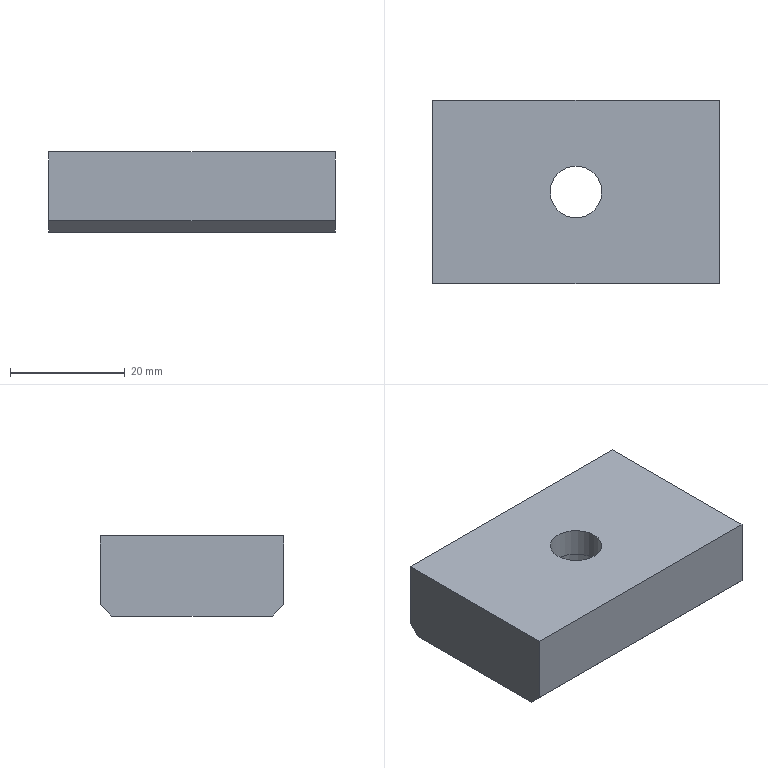Part | NX | features solid 2 | 1 solid | 11 faces | box 50 x 32 x 14 mm | volume 20496 mm3 | plane 9 | cylinder 2 | commonest cylinder face diameters 9 x1 14 x1
STEP:
#1=CARTESIAN_POINT('',(-210.,-250.,137.));
#2=VERTEX_POINT('',#1);
#3=CARTESIAN_POINT('',(-210.,-250.,149.));
#4=VERTEX_POINT('',#3);
#5=CARTESIAN_POINT('',(-210.,-250.,135.));
#6=DIRECTION('',(0.,0.,1.));
#7=VECTOR('',#6,1000.);
#8=LINE('',#5,#7);
#9=EDGE_CURVE('',#2,#4,#8,.T.);
#10=ORIENTED_EDGE('',*,*,#9,.F.);
#11=CARTESIAN_POINT('',(-260.,-250.,137.));
#12=VERTEX_POINT('',#11);
#13=CARTESIAN_POINT('',(-260.,-250.,137.));
#14=DIRECTION('',(-1.,0.,0.));
#15=VECTOR('',#14,1000.);
#16=LINE('',#13,#15);
#17=EDGE_CURVE('',#2,#12,#16,.T.);
#18=ORIENTED_EDGE('',*,*,#17,.T.);
#19=CARTESIAN_POINT('',(-260.,-250.,149.));
#20=VERTEX_POINT('',#19);
#21=CARTESIAN_POINT('',(-260.,-250.,135.));
#22=DIRECTION('',(0.,0.,1.));
#23=VECTOR('',#22,1000.);
#24=LINE('',#21,#23);
#25=EDGE_CURVE('',#12,#20,#24,.T.);
#26=ORIENTED_EDGE('',*,*,#25,.T.);
#27=CARTESIAN_POINT('',(-260.,-250.,149.));
#28=DIRECTION('',(-1.,0.,0.));
#29=VECTOR('',#28,1000.);
#30=LINE('',#27,#29);
#31=EDGE_CURVE('',#20,#4,#30,.F.);
#32=ORIENTED_EDGE('',*,*,#31,.T.);
#33=EDGE_LOOP('',(#10,#18,#26,#32));
#34=FACE_BOUND('',#33,.T.);
#35=CARTESIAN_POINT('',(-260.,-250.,135.));
#36=DIRECTION('',(0.,1.,0.));
#37=DIRECTION('',(1.,0.,0.));
#38=AXIS2_PLACEMENT_3D('',#35,#36,#37);
#39=PLANE('',#38);
#40=ADVANCED_FACE('',(#34),#39,.T.);
#41=ORIENTED_EDGE('',*,*,#25,.F.);
#42=CARTESIAN_POINT('',(-260.,-252.,135.));
#43=VERTEX_POINT('',#42);
#44=CARTESIAN_POINT('',(-260.,-251.,136.));
#45=DIRECTION('',(0.,-0.7071,-0.7071));
#46=VECTOR('',#45,1000.);
#47=LINE('',#44,#46);
#48=EDGE_CURVE('',#12,#43,#47,.T.);
#49=ORIENTED_EDGE('',*,*,#48,.T.);
#50=CARTESIAN_POINT('',(-260.,-280.,135.));
#51=VERTEX_POINT('',#50);
#52=CARTESIAN_POINT('',(-260.,-256.,135.));
#53=DIRECTION('',(0.,-1.,0.));
#54=VECTOR('',#53,1000.);
#55=LINE('',#52,#54);
#56=EDGE_CURVE('',#43,#51,#55,.T.);
#57=ORIENTED_EDGE('',*,*,#56,.T.);
#58=CARTESIAN_POINT('',(-260.,-282.,137.));
#59=VERTEX_POINT('',#58);
#60=CARTESIAN_POINT('',(-260.,-271.,126.));
#61=DIRECTION('',(0.,0.7071,-0.7071));
#62=VECTOR('',#61,1000.);
#63=LINE('',#60,#62);
#64=EDGE_CURVE('',#51,#59,#63,.F.);
#65=ORIENTED_EDGE('',*,*,#64,.T.);
#66=CARTESIAN_POINT('',(-260.,-282.,149.));
#67=VERTEX_POINT('',#66);
#68=CARTESIAN_POINT('',(-260.,-282.,135.));
#69=DIRECTION('',(0.,0.,1.));
#70=VECTOR('',#69,1000.);
#71=LINE('',#68,#70);
#72=EDGE_CURVE('',#59,#67,#71,.T.);
#73=ORIENTED_EDGE('',*,*,#72,.T.);
#74=CARTESIAN_POINT('',(-260.,-256.,149.));
#75=DIRECTION('',(0.,1.,0.));
#76=VECTOR('',#75,1000.);
#77=LINE('',#74,#76);
#78=EDGE_CURVE('',#20,#67,#77,.F.);
#79=ORIENTED_EDGE('',*,*,#78,.F.);
#80=EDGE_LOOP('',(#41,#49,#57,#65,#73,#79));
#81=FACE_BOUND('',#80,.T.);
#82=CARTESIAN_POINT('',(-260.,-256.,135.));
#83=DIRECTION('',(1.,0.,0.));
#84=DIRECTION('',(0.,-1.,0.));
#85=AXIS2_PLACEMENT_3D('',#82,#83,#84);
#86=PLANE('',#85);
#87=ADVANCED_FACE('',(#81),#86,.F.);
#88=ORIENTED_EDGE('',*,*,#72,.F.);
#89=CARTESIAN_POINT('',(-210.,-282.,137.));
#90=VERTEX_POINT('',#89);
#91=CARTESIAN_POINT('',(-260.,-282.,137.));
#92=DIRECTION('',(-1.,0.,0.));
#93=VECTOR('',#92,1000.);
#94=LINE('',#91,#93);
#95=EDGE_CURVE('',#59,#90,#94,.F.);
#96=ORIENTED_EDGE('',*,*,#95,.T.);
#97=CARTESIAN_POINT('',(-210.,-282.,149.));
#98=VERTEX_POINT('',#97);
#99=CARTESIAN_POINT('',(-210.,-282.,135.));
#100=DIRECTION('',(0.,0.,1.));
#101=VECTOR('',#100,1000.);
#102=LINE('',#99,#101);
#103=EDGE_CURVE('',#90,#98,#102,.T.);
#104=ORIENTED_EDGE('',*,*,#103,.T.);
#105=CARTESIAN_POINT('',(-260.,-282.,149.));
#106=DIRECTION('',(-1.,0.,0.));
#107=VECTOR('',#106,1000.);
#108=LINE('',#105,#107);
#109=EDGE_CURVE('',#67,#98,#108,.F.);
#110=ORIENTED_EDGE('',*,*,#109,.F.);
#111=EDGE_LOOP('',(#88,#96,#104,#110));
#112=FACE_BOUND('',#111,.T.);
#113=CARTESIAN_POINT('',(-260.,-282.,135.));
#114=DIRECTION('',(0.,1.,0.));
#115=DIRECTION('',(1.,0.,0.));
#116=AXIS2_PLACEMENT_3D('',#113,#114,#115);
#117=PLANE('',#116);
#118=ADVANCED_FACE('',(#112),#117,.F.);
#119=CARTESIAN_POINT('',(-239.5,-266.,149.));
#120=VERTEX_POINT('',#119);
#121=CARTESIAN_POINT('',(-235.,-266.,149.));
#122=DIRECTION('',(0.,0.,-1.));
#123=DIRECTION('',(-1.,0.,0.));
#124=AXIS2_PLACEMENT_3D('',#121,#122,#123);
#125=CIRCLE('',#124,4.5);
#126=EDGE_CURVE('',#120,#120,#125,.T.);
#127=ORIENTED_EDGE('',*,*,#126,.T.);
#128=EDGE_LOOP('',(#127));
#129=FACE_BOUND('',#128,.T.);
#130=ORIENTED_EDGE('',*,*,#109,.T.);
#131=CARTESIAN_POINT('',(-210.,-256.,149.));
#132=DIRECTION('',(0.,1.,0.));
#133=VECTOR('',#132,1000.);
#134=LINE('',#131,#133);
#135=EDGE_CURVE('',#4,#98,#134,.F.);
#136=ORIENTED_EDGE('',*,*,#135,.F.);
#137=ORIENTED_EDGE('',*,*,#31,.F.);
#138=ORIENTED_EDGE('',*,*,#78,.T.);
#139=EDGE_LOOP('',(#130,#136,#137,#138));
#140=FACE_BOUND('',#139,.T.);
#141=CARTESIAN_POINT('',(-260.,-256.,149.));
#142=DIRECTION('',(0.,0.,-1.));
#143=DIRECTION('',(-1.,0.,0.));
#144=AXIS2_PLACEMENT_3D('',#141,#142,#143);
#145=PLANE('',#144);
#146=ADVANCED_FACE('',(#129,#140),#145,.F.);
#147=CARTESIAN_POINT('',(-210.,-252.,135.));
#148=VERTEX_POINT('',#147);
#149=CARTESIAN_POINT('',(-210.,-280.,135.));
#150=VERTEX_POINT('',#149);
#151=CARTESIAN_POINT('',(-210.,-256.,135.));
#152=DIRECTION('',(0.,-1.,0.));
#153=VECTOR('',#152,1000.);
#154=LINE('',#151,#153);
#155=EDGE_CURVE('',#148,#150,#154,.T.);
#156=ORIENTED_EDGE('',*,*,#155,.F.);
#157=CARTESIAN_POINT('',(-210.,-251.,136.));
#158=DIRECTION('',(0.,-0.7071,-0.7071));
#159=VECTOR('',#158,1000.);
#160=LINE('',#157,#159);
#161=EDGE_CURVE('',#148,#2,#160,.F.);
#162=ORIENTED_EDGE('',*,*,#161,.T.);
#163=ORIENTED_EDGE('',*,*,#9,.T.);
#164=ORIENTED_EDGE('',*,*,#135,.T.);
#165=ORIENTED_EDGE('',*,*,#103,.F.);
#166=CARTESIAN_POINT('',(-210.,-271.,126.));
#167=DIRECTION('',(0.,0.7071,-0.7071));
#168=VECTOR('',#167,1000.);
#169=LINE('',#166,#168);
#170=EDGE_CURVE('',#90,#150,#169,.T.);
#171=ORIENTED_EDGE('',*,*,#170,.T.);
#172=EDGE_LOOP('',(#156,#162,#163,#164,#165,#171));
#173=FACE_BOUND('',#172,.T.);
#174=CARTESIAN_POINT('',(-210.,-256.,135.));
#175=DIRECTION('',(1.,0.,0.));
#176=DIRECTION('',(0.,-1.,0.));
#177=AXIS2_PLACEMENT_3D('',#174,#175,#176);
#178=PLANE('',#177);
#179=ADVANCED_FACE('',(#173),#178,.T.);
#180=CARTESIAN_POINT('',(-228.,-266.,135.));
#181=VERTEX_POINT('',#180);
#182=CARTESIAN_POINT('',(-235.,-266.,135.));
#183=DIRECTION('',(0.,0.,1.));
#184=DIRECTION('',(1.,0.,0.));
#185=AXIS2_PLACEMENT_3D('',#182,#183,#184);
#186=CIRCLE('',#185,7.);
#187=EDGE_CURVE('',#181,#181,#186,.T.);
#188=ORIENTED_EDGE('',*,*,#187,.T.);
#189=EDGE_LOOP('',(#188));
#190=FACE_BOUND('',#189,.T.);
#191=ORIENTED_EDGE('',*,*,#56,.F.);
#192=CARTESIAN_POINT('',(-260.,-252.,135.));
#193=DIRECTION('',(1.,0.,0.));
#194=VECTOR('',#193,1000.);
#195=LINE('',#192,#194);
#196=EDGE_CURVE('',#43,#148,#195,.T.);
#197=ORIENTED_EDGE('',*,*,#196,.T.);
#198=ORIENTED_EDGE('',*,*,#155,.T.);
#199=CARTESIAN_POINT('',(-260.,-280.,135.));
#200=DIRECTION('',(-1.,0.,0.));
#201=VECTOR('',#200,1000.);
#202=LINE('',#199,#201);
#203=EDGE_CURVE('',#150,#51,#202,.T.);
#204=ORIENTED_EDGE('',*,*,#203,.T.);
#205=EDGE_LOOP('',(#191,#197,#198,#204));
#206=FACE_BOUND('',#205,.T.);
#207=CARTESIAN_POINT('',(-260.,-256.,135.));
#208=DIRECTION('',(0.,0.,-1.));
#209=DIRECTION('',(-1.,0.,0.));
#210=AXIS2_PLACEMENT_3D('',#207,#208,#209);
#211=PLANE('',#210);
#212=ADVANCED_FACE('',(#190,#206),#211,.T.);
#213=ORIENTED_EDGE('',*,*,#48,.F.);
#214=ORIENTED_EDGE('',*,*,#17,.F.);
#215=ORIENTED_EDGE('',*,*,#161,.F.);
#216=ORIENTED_EDGE('',*,*,#196,.F.);
#217=EDGE_LOOP('',(#213,#214,#215,#216));
#218=FACE_BOUND('',#217,.T.);
#219=CARTESIAN_POINT('',(-260.,-252.,135.));
#220=DIRECTION('',(0.,-0.7071,0.7071));
#221=DIRECTION('',(0.,-0.7071,-0.7071));
#222=AXIS2_PLACEMENT_3D('',#219,#220,#221);
#223=PLANE('',#222);
#224=ADVANCED_FACE('',(#218),#223,.F.);
#225=ORIENTED_EDGE('',*,*,#64,.F.);
#226=ORIENTED_EDGE('',*,*,#203,.F.);
#227=ORIENTED_EDGE('',*,*,#170,.F.);
#228=ORIENTED_EDGE('',*,*,#95,.F.);
#229=EDGE_LOOP('',(#225,#226,#227,#228));
#230=FACE_BOUND('',#229,.T.);
#231=CARTESIAN_POINT('',(-260.,-282.,137.));
#232=DIRECTION('',(0.,-0.7071,-0.7071));
#233=DIRECTION('',(0.,0.7071,-0.7071));
#234=AXIS2_PLACEMENT_3D('',#231,#232,#233);
#235=PLANE('',#234);
#236=ADVANCED_FACE('',(#230),#235,.T.);
#237=ORIENTED_EDGE('',*,*,#187,.F.);
#238=EDGE_LOOP('',(#237));
#239=FACE_BOUND('',#238,.T.);
#240=CARTESIAN_POINT('',(-228.,-266.,144.));
#241=VERTEX_POINT('',#240);
#242=CARTESIAN_POINT('',(-235.,-266.,144.));
#243=DIRECTION('',(0.,0.,1.));
#244=DIRECTION('',(1.,0.,0.));
#245=AXIS2_PLACEMENT_3D('',#242,#243,#244);
#246=CIRCLE('',#245,7.);
#247=EDGE_CURVE('',#241,#241,#246,.T.);
#248=ORIENTED_EDGE('',*,*,#247,.T.);
#249=EDGE_LOOP('',(#248));
#250=FACE_BOUND('',#249,.T.);
#251=CARTESIAN_POINT('',(-235.,-266.,135.));
#252=DIRECTION('',(0.,0.,1.));
#253=DIRECTION('',(1.,0.,0.));
#254=AXIS2_PLACEMENT_3D('',#251,#252,#253);
#255=CYLINDRICAL_SURFACE('',#254,7.);
#256=ADVANCED_FACE('',(#239,#250),#255,.F.);
#257=CARTESIAN_POINT('',(-230.5,-266.,144.));
#258=VERTEX_POINT('',#257);
#259=CARTESIAN_POINT('',(-235.,-266.,144.));
#260=DIRECTION('',(0.,0.,1.));
#261=DIRECTION('',(1.,0.,0.));
#262=AXIS2_PLACEMENT_3D('',#259,#260,#261);
#263=CIRCLE('',#262,4.5);
#264=EDGE_CURVE('',#258,#258,#263,.T.);
#265=ORIENTED_EDGE('',*,*,#264,.T.);
#266=EDGE_LOOP('',(#265));
#267=FACE_BOUND('',#266,.T.);
#268=ORIENTED_EDGE('',*,*,#247,.F.);
#269=EDGE_LOOP('',(#268));
#270=FACE_BOUND('',#269,.T.);
#271=CARTESIAN_POINT('',(-235.,-266.,144.));
#272=DIRECTION('',(0.,0.,1.));
#273=DIRECTION('',(1.,0.,0.));
#274=AXIS2_PLACEMENT_3D('',#271,#272,#273);
#275=PLANE('',#274);
#276=ADVANCED_FACE('',(#267,#270),#275,.F.);
#277=ORIENTED_EDGE('',*,*,#264,.F.);
#278=EDGE_LOOP('',(#277));
#279=FACE_BOUND('',#278,.T.);
#280=ORIENTED_EDGE('',*,*,#126,.F.);
#281=EDGE_LOOP('',(#280));
#282=FACE_BOUND('',#281,.T.);
#283=CARTESIAN_POINT('',(-235.,-266.,135.));
#284=DIRECTION('',(0.,0.,1.));
#285=DIRECTION('',(1.,0.,0.));
#286=AXIS2_PLACEMENT_3D('',#283,#284,#285);
#287=CYLINDRICAL_SURFACE('',#286,4.5);
#288=ADVANCED_FACE('',(#279,#282),#287,.F.);
#289=CLOSED_SHELL('',(#40,#87,#118,#146,#179,#212,#224,#236,#256,#276,#288));
#290=MANIFOLD_SOLID_BREP('',#289);
#291=(LENGTH_UNIT()NAMED_UNIT(*)SI_UNIT(.MILLI.,.METRE.));
#292=UNCERTAINTY_MEASURE_WITH_UNIT(LENGTH_MEASURE(0.00001),#291,'','');
#293=(NAMED_UNIT(*)PLANE_ANGLE_UNIT()SI_UNIT($,.RADIAN.));
#294=(NAMED_UNIT(*)SI_UNIT($,.STERADIAN.)SOLID_ANGLE_UNIT());
#295=(GEOMETRIC_REPRESENTATION_CONTEXT(3)GLOBAL_UNCERTAINTY_ASSIGNED_CONTEXT((#292))GLOBAL_UNIT_ASSIGNED_CONTEXT((#291,#293,#294))REPRESENTATION_CONTEXT('',''));
#296=ADVANCED_BREP_SHAPE_REPRESENTATION('',(#290),#295);